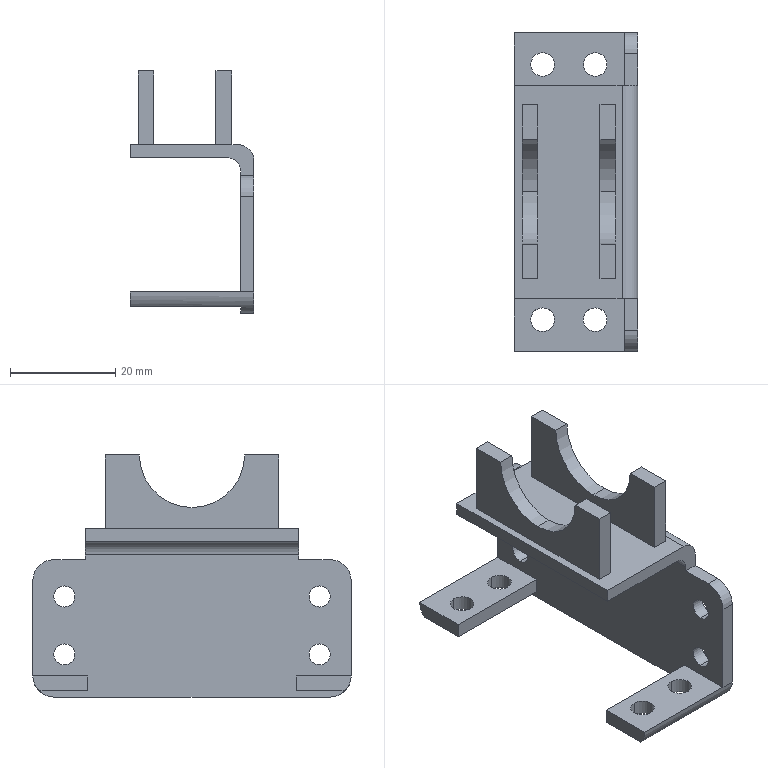Part | SolidWorks | features ICE 4, Cut 3, Fillet 2, MirrorPattern 2, Extrusion 1 | 1 solid | 58 faces | box 23.5 x 60.5 x 46 mm | volume 9322 mm3 | plane 32 | cylinder 26 | commonest cylinder face diameters 4 x8 4.5 x8 8 x4 20 x4 5 x1 6 x1